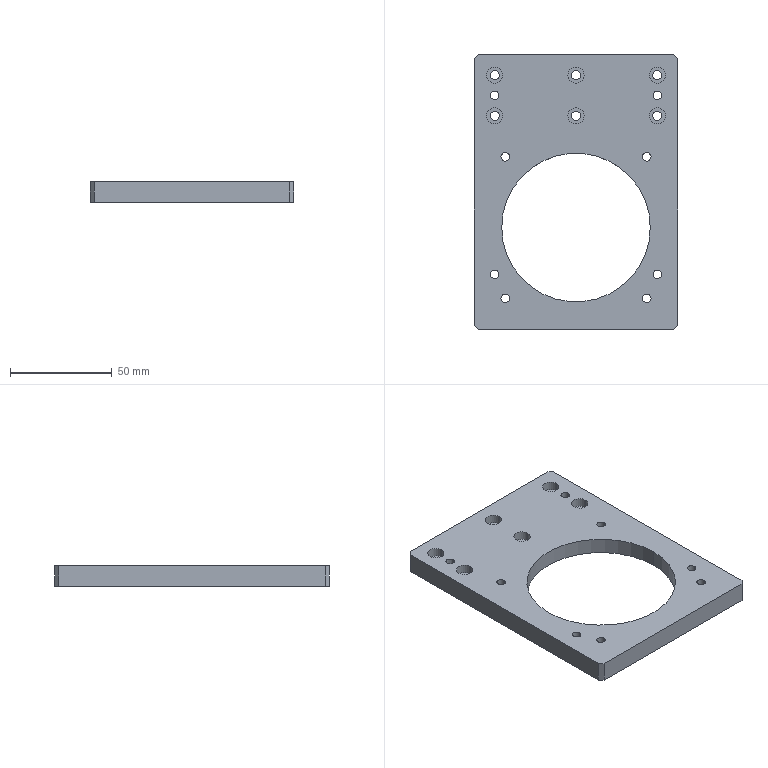Part | STEP file | PN_0008 | 1 solid | 67 faces | box 100 x 135 x 10 mm | volume 83048 mm3 | cylinder 46 | plane 21 | commonest cylinder face diameters 4.2 x16 4.5 x12 8 x12 6 x4 73.1 x2